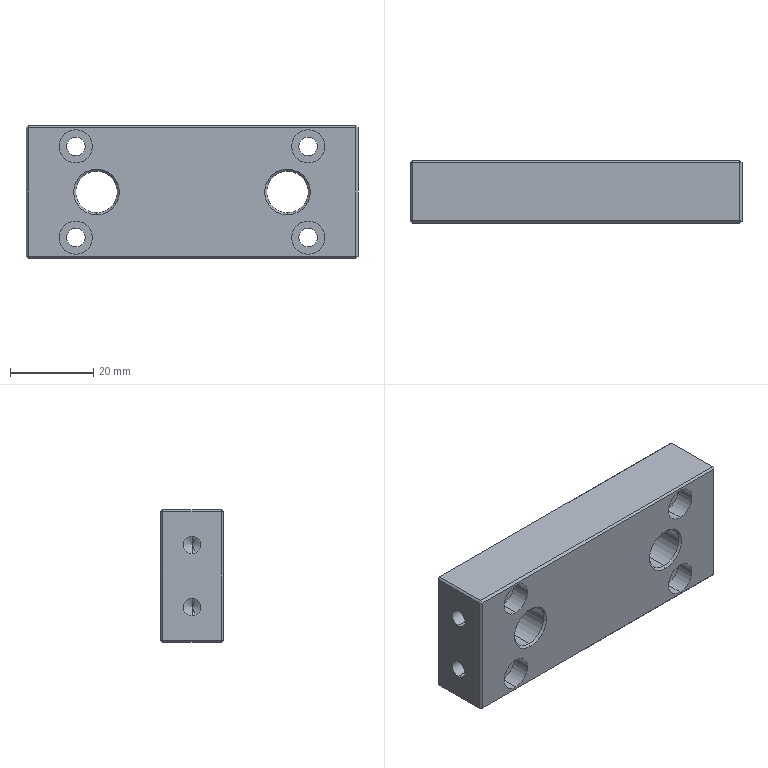Part | SolidWorks | features HoleWzd 3, Chamfer 1, Cut 1, ExtruThin 1 | 1 solid | 74 faces | box 80 x 15 x 32 mm | volume 33801 mm3 | plane 30 | cylinder 28 | cone 16 | commonest cylinder face diameters 4.2 x8 4.5 x8 8 x8 10 x4